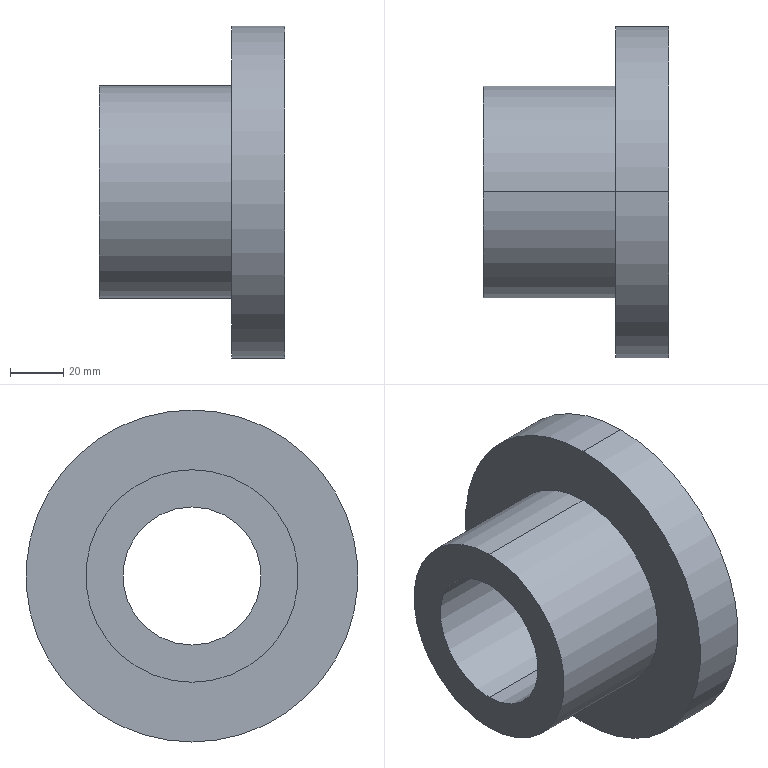Part | SolidWorks | features Revolution 1 | 1 solid | 9 faces | box 70 x 125 x 125 mm | volume 348104 mm3 | cylinder 6 | plane 3 | commonest cylinder face diameters 52 x2 80 x2 125 x2
STEP:
#1=CARTESIAN_POINT('',(70.,0.,62.5));
#2=VERTEX_POINT('',#1);
#3=CARTESIAN_POINT('',(70.,0.,-62.5));
#4=VERTEX_POINT('',#3);
#5=CARTESIAN_POINT('',(70.,0.,0.));
#6=DIRECTION('',(-1.,0.,0.));
#7=DIRECTION('',(0.,0.,1.));
#8=AXIS2_PLACEMENT_3D('',#5,#6,#7);
#9=CIRCLE('',#8,62.5);
#10=EDGE_CURVE('',#2,#4,#9,.T.);
#11=ORIENTED_EDGE('',*,*,#10,.T.);
#12=CARTESIAN_POINT('',(50.,0.,-62.5));
#13=VERTEX_POINT('',#12);
#14=CARTESIAN_POINT('',(0.,0.,-62.5));
#15=DIRECTION('',(-1.,0.,0.));
#16=VECTOR('',#15,1000.);
#17=LINE('',#14,#16);
#18=EDGE_CURVE('',#4,#13,#17,.T.);
#19=ORIENTED_EDGE('',*,*,#18,.T.);
#20=CARTESIAN_POINT('',(50.,0.,62.5));
#21=VERTEX_POINT('',#20);
#22=CARTESIAN_POINT('',(50.,0.,0.));
#23=DIRECTION('',(-1.,0.,0.));
#24=DIRECTION('',(0.,0.,1.));
#25=AXIS2_PLACEMENT_3D('',#22,#23,#24);
#26=CIRCLE('',#25,62.5);
#27=EDGE_CURVE('',#21,#13,#26,.T.);
#28=ORIENTED_EDGE('',*,*,#27,.F.);
#29=CARTESIAN_POINT('',(0.,0.,62.5));
#30=DIRECTION('',(-1.,0.,0.));
#31=VECTOR('',#30,1000.);
#32=LINE('',#29,#31);
#33=EDGE_CURVE('',#2,#21,#32,.T.);
#34=ORIENTED_EDGE('',*,*,#33,.F.);
#35=EDGE_LOOP('',(#11,#19,#28,#34));
#36=FACE_OUTER_BOUND('',#35,.T.);
#37=CARTESIAN_POINT('',(0.,0.,0.));
#38=DIRECTION('',(-1.,0.,0.));
#39=DIRECTION('',(0.,0.,1.));
#40=AXIS2_PLACEMENT_3D('',#37,#38,#39);
#41=CYLINDRICAL_SURFACE('',#40,62.5);
#42=ADVANCED_FACE('',(#36),#41,.T.);
#43=CARTESIAN_POINT('',(50.,0.,40.));
#44=VERTEX_POINT('',#43);
#45=CARTESIAN_POINT('',(50.,0.,-40.));
#46=VERTEX_POINT('',#45);
#47=CARTESIAN_POINT('',(50.,0.,0.));
#48=DIRECTION('',(-1.,0.,0.));
#49=DIRECTION('',(0.,0.,1.));
#50=AXIS2_PLACEMENT_3D('',#47,#48,#49);
#51=CIRCLE('',#50,40.);
#52=EDGE_CURVE('',#44,#46,#51,.T.);
#53=ORIENTED_EDGE('',*,*,#52,.T.);
#54=CARTESIAN_POINT('',(0.,0.,-40.));
#55=VERTEX_POINT('',#54);
#56=CARTESIAN_POINT('',(0.,0.,-40.));
#57=DIRECTION('',(-1.,0.,0.));
#58=VECTOR('',#57,1000.);
#59=LINE('',#56,#58);
#60=EDGE_CURVE('',#46,#55,#59,.T.);
#61=ORIENTED_EDGE('',*,*,#60,.T.);
#62=CARTESIAN_POINT('',(0.,0.,40.));
#63=VERTEX_POINT('',#62);
#64=CARTESIAN_POINT('',(0.,0.,0.));
#65=DIRECTION('',(-1.,0.,0.));
#66=DIRECTION('',(0.,0.,1.));
#67=AXIS2_PLACEMENT_3D('',#64,#65,#66);
#68=CIRCLE('',#67,40.);
#69=EDGE_CURVE('',#63,#55,#68,.T.);
#70=ORIENTED_EDGE('',*,*,#69,.F.);
#71=CARTESIAN_POINT('',(0.,0.,40.));
#72=DIRECTION('',(-1.,0.,0.));
#73=VECTOR('',#72,1000.);
#74=LINE('',#71,#73);
#75=EDGE_CURVE('',#44,#63,#74,.T.);
#76=ORIENTED_EDGE('',*,*,#75,.F.);
#77=EDGE_LOOP('',(#53,#61,#70,#76));
#78=FACE_OUTER_BOUND('',#77,.T.);
#79=CARTESIAN_POINT('',(0.,0.,0.));
#80=DIRECTION('',(-1.,0.,0.));
#81=DIRECTION('',(0.,0.,1.));
#82=AXIS2_PLACEMENT_3D('',#79,#80,#81);
#83=CYLINDRICAL_SURFACE('',#82,40.);
#84=ADVANCED_FACE('',(#78),#83,.T.);
#85=CARTESIAN_POINT('',(70.,0.,-26.));
#86=VERTEX_POINT('',#85);
#87=CARTESIAN_POINT('',(70.,0.,26.));
#88=VERTEX_POINT('',#87);
#89=CARTESIAN_POINT('',(70.,0.,0.));
#90=DIRECTION('',(-1.,0.,0.));
#91=DIRECTION('',(0.,0.,1.));
#92=AXIS2_PLACEMENT_3D('',#89,#90,#91);
#93=CIRCLE('',#92,26.);
#94=EDGE_CURVE('',#86,#88,#93,.T.);
#95=ORIENTED_EDGE('',*,*,#94,.F.);
#96=CARTESIAN_POINT('',(0.,0.,-26.));
#97=VERTEX_POINT('',#96);
#98=CARTESIAN_POINT('',(0.,0.,-26.));
#99=DIRECTION('',(-1.,0.,0.));
#100=VECTOR('',#99,1000.);
#101=LINE('',#98,#100);
#102=EDGE_CURVE('',#86,#97,#101,.T.);
#103=ORIENTED_EDGE('',*,*,#102,.T.);
#104=CARTESIAN_POINT('',(0.,0.,26.));
#105=VERTEX_POINT('',#104);
#106=CARTESIAN_POINT('',(0.,0.,0.));
#107=DIRECTION('',(-1.,0.,0.));
#108=DIRECTION('',(0.,0.,1.));
#109=AXIS2_PLACEMENT_3D('',#106,#107,#108);
#110=CIRCLE('',#109,26.);
#111=EDGE_CURVE('',#97,#105,#110,.T.);
#112=ORIENTED_EDGE('',*,*,#111,.T.);
#113=CARTESIAN_POINT('',(0.,0.,26.));
#114=DIRECTION('',(-1.,0.,0.));
#115=VECTOR('',#114,1000.);
#116=LINE('',#113,#115);
#117=EDGE_CURVE('',#88,#105,#116,.T.);
#118=ORIENTED_EDGE('',*,*,#117,.F.);
#119=EDGE_LOOP('',(#95,#103,#112,#118));
#120=FACE_OUTER_BOUND('',#119,.T.);
#121=CARTESIAN_POINT('',(0.,0.,0.));
#122=DIRECTION('',(-1.,0.,0.));
#123=DIRECTION('',(0.,0.,1.));
#124=AXIS2_PLACEMENT_3D('',#121,#122,#123);
#125=CYLINDRICAL_SURFACE('',#124,26.);
#126=ADVANCED_FACE('',(#120),#125,.F.);
#127=ORIENTED_EDGE('',*,*,#102,.F.);
#128=CARTESIAN_POINT('',(70.,0.,0.));
#129=DIRECTION('',(-1.,0.,0.));
#130=DIRECTION('',(0.,0.,1.));
#131=AXIS2_PLACEMENT_3D('',#128,#129,#130);
#132=CIRCLE('',#131,26.);
#133=EDGE_CURVE('',#88,#86,#132,.T.);
#134=ORIENTED_EDGE('',*,*,#133,.F.);
#135=ORIENTED_EDGE('',*,*,#117,.T.);
#136=CARTESIAN_POINT('',(0.,0.,0.));
#137=DIRECTION('',(-1.,0.,0.));
#138=DIRECTION('',(0.,0.,1.));
#139=AXIS2_PLACEMENT_3D('',#136,#137,#138);
#140=CIRCLE('',#139,26.);
#141=EDGE_CURVE('',#105,#97,#140,.T.);
#142=ORIENTED_EDGE('',*,*,#141,.T.);
#143=EDGE_LOOP('',(#127,#134,#135,#142));
#144=FACE_OUTER_BOUND('',#143,.T.);
#145=CARTESIAN_POINT('',(0.,0.,0.));
#146=DIRECTION('',(-1.,0.,0.));
#147=DIRECTION('',(0.,0.,1.));
#148=AXIS2_PLACEMENT_3D('',#145,#146,#147);
#149=CYLINDRICAL_SURFACE('',#148,26.);
#150=ADVANCED_FACE('',(#144),#149,.F.);
#151=ORIENTED_EDGE('',*,*,#69,.T.);
#152=CARTESIAN_POINT('',(0.,0.,0.));
#153=DIRECTION('',(-1.,0.,0.));
#154=DIRECTION('',(0.,0.,1.));
#155=AXIS2_PLACEMENT_3D('',#152,#153,#154);
#156=CIRCLE('',#155,40.);
#157=EDGE_CURVE('',#55,#63,#156,.T.);
#158=ORIENTED_EDGE('',*,*,#157,.T.);
#159=EDGE_LOOP('',(#151,#158));
#160=FACE_OUTER_BOUND('',#159,.T.);
#161=ORIENTED_EDGE('',*,*,#141,.F.);
#162=ORIENTED_EDGE('',*,*,#111,.F.);
#163=EDGE_LOOP('',(#161,#162));
#164=FACE_BOUND('',#163,.T.);
#165=CARTESIAN_POINT('',(0.,-26.,0.));
#166=DIRECTION('',(-1.,0.,0.));
#167=DIRECTION('',(0.,0.,1.));
#168=AXIS2_PLACEMENT_3D('',#165,#166,#167);
#169=PLANE('',#168);
#170=ADVANCED_FACE('',(#160,#164),#169,.T.);
#171=ORIENTED_EDGE('',*,*,#60,.F.);
#172=CARTESIAN_POINT('',(50.,0.,0.));
#173=DIRECTION('',(-1.,0.,0.));
#174=DIRECTION('',(0.,0.,1.));
#175=AXIS2_PLACEMENT_3D('',#172,#173,#174);
#176=CIRCLE('',#175,40.);
#177=EDGE_CURVE('',#46,#44,#176,.T.);
#178=ORIENTED_EDGE('',*,*,#177,.T.);
#179=ORIENTED_EDGE('',*,*,#75,.T.);
#180=ORIENTED_EDGE('',*,*,#157,.F.);
#181=EDGE_LOOP('',(#171,#178,#179,#180));
#182=FACE_OUTER_BOUND('',#181,.T.);
#183=CARTESIAN_POINT('',(0.,0.,0.));
#184=DIRECTION('',(-1.,0.,0.));
#185=DIRECTION('',(0.,0.,1.));
#186=AXIS2_PLACEMENT_3D('',#183,#184,#185);
#187=CYLINDRICAL_SURFACE('',#186,40.);
#188=ADVANCED_FACE('',(#182),#187,.T.);
#189=ORIENTED_EDGE('',*,*,#27,.T.);
#190=CARTESIAN_POINT('',(50.,0.,0.));
#191=DIRECTION('',(-1.,0.,0.));
#192=DIRECTION('',(0.,0.,1.));
#193=AXIS2_PLACEMENT_3D('',#190,#191,#192);
#194=CIRCLE('',#193,62.5);
#195=EDGE_CURVE('',#13,#21,#194,.T.);
#196=ORIENTED_EDGE('',*,*,#195,.T.);
#197=EDGE_LOOP('',(#189,#196));
#198=FACE_OUTER_BOUND('',#197,.T.);
#199=ORIENTED_EDGE('',*,*,#52,.F.);
#200=ORIENTED_EDGE('',*,*,#177,.F.);
#201=EDGE_LOOP('',(#199,#200));
#202=FACE_BOUND('',#201,.T.);
#203=CARTESIAN_POINT('',(50.,-40.,0.));
#204=DIRECTION('',(-1.,0.,0.));
#205=DIRECTION('',(0.,0.,1.));
#206=AXIS2_PLACEMENT_3D('',#203,#204,#205);
#207=PLANE('',#206);
#208=ADVANCED_FACE('',(#198,#202),#207,.T.);
#209=ORIENTED_EDGE('',*,*,#18,.F.);
#210=CARTESIAN_POINT('',(70.,0.,0.));
#211=DIRECTION('',(-1.,0.,0.));
#212=DIRECTION('',(0.,0.,1.));
#213=AXIS2_PLACEMENT_3D('',#210,#211,#212);
#214=CIRCLE('',#213,62.5);
#215=EDGE_CURVE('',#4,#2,#214,.T.);
#216=ORIENTED_EDGE('',*,*,#215,.T.);
#217=ORIENTED_EDGE('',*,*,#33,.T.);
#218=ORIENTED_EDGE('',*,*,#195,.F.);
#219=EDGE_LOOP('',(#209,#216,#217,#218));
#220=FACE_OUTER_BOUND('',#219,.T.);
#221=CARTESIAN_POINT('',(0.,0.,0.));
#222=DIRECTION('',(-1.,0.,0.));
#223=DIRECTION('',(0.,0.,1.));
#224=AXIS2_PLACEMENT_3D('',#221,#222,#223);
#225=CYLINDRICAL_SURFACE('',#224,62.5);
#226=ADVANCED_FACE('',(#220),#225,.T.);
#227=ORIENTED_EDGE('',*,*,#133,.T.);
#228=ORIENTED_EDGE('',*,*,#94,.T.);
#229=EDGE_LOOP('',(#227,#228));
#230=FACE_BOUND('',#229,.T.);
#231=ORIENTED_EDGE('',*,*,#10,.F.);
#232=ORIENTED_EDGE('',*,*,#215,.F.);
#233=EDGE_LOOP('',(#231,#232));
#234=FACE_OUTER_BOUND('',#233,.T.);
#235=CARTESIAN_POINT('',(70.,-62.5,0.));
#236=DIRECTION('',(1.,0.,0.));
#237=DIRECTION('',(0.,0.,-1.));
#238=AXIS2_PLACEMENT_3D('',#235,#236,#237);
#239=PLANE('',#238);
#240=ADVANCED_FACE('',(#230,#234),#239,.T.);
#241=CLOSED_SHELL('',(#42,#84,#126,#150,#170,#188,#208,#226,#240));
#242=MANIFOLD_SOLID_BREP('',#241);
#243=CARTESIAN_POINT('',(0.,0.,0.));
#244=DIRECTION('',(0.,0.,1.));
#245=DIRECTION('',(1.,0.,0.));
#246=AXIS2_PLACEMENT_3D('',#243,#244,#245);
#247=(LENGTH_UNIT()NAMED_UNIT(*)SI_UNIT(.MILLI.,.METRE.));
#248=UNCERTAINTY_MEASURE_WITH_UNIT(LENGTH_MEASURE(0.00001),#247,'','');
#249=(NAMED_UNIT(*)PLANE_ANGLE_UNIT()SI_UNIT($,.RADIAN.));
#250=(NAMED_UNIT(*)SI_UNIT($,.STERADIAN.)SOLID_ANGLE_UNIT());
#251=(GEOMETRIC_REPRESENTATION_CONTEXT(3)GLOBAL_UNCERTAINTY_ASSIGNED_CONTEXT((#248))GLOBAL_UNIT_ASSIGNED_CONTEXT((#247,#249,#250))REPRESENTATION_CONTEXT('',''));
#252=ADVANCED_BREP_SHAPE_REPRESENTATION('',(#242,#246),#251);